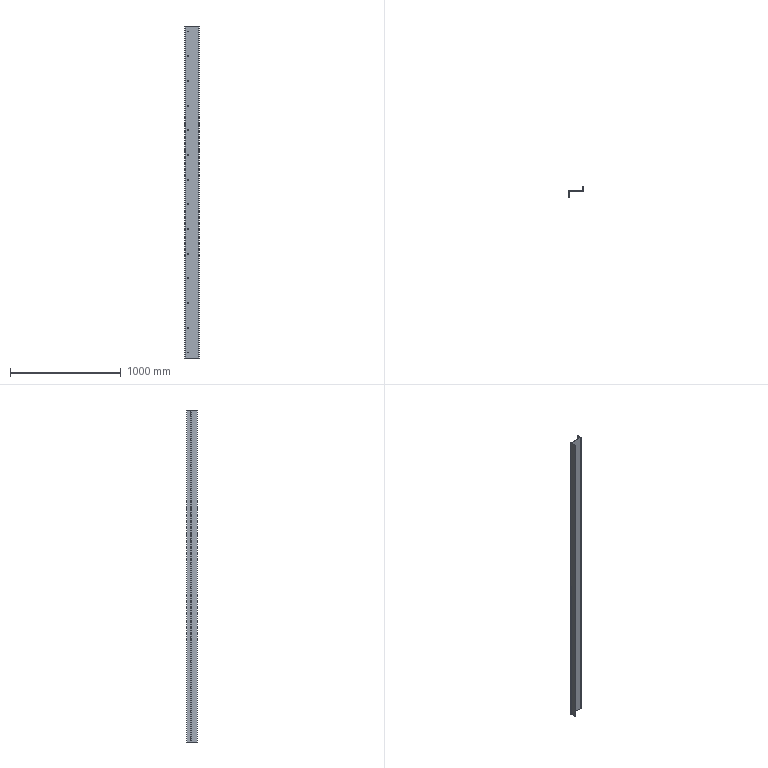Part | STEP file | SX-Z001-01 | 1 solid | 50 faces | box 131 x 95 x 2995 mm | volume 1988432 mm3 | cylinder 32 | plane 18 | commonest cylinder face diameters 8 x28 0.4 x2 6.4 x2